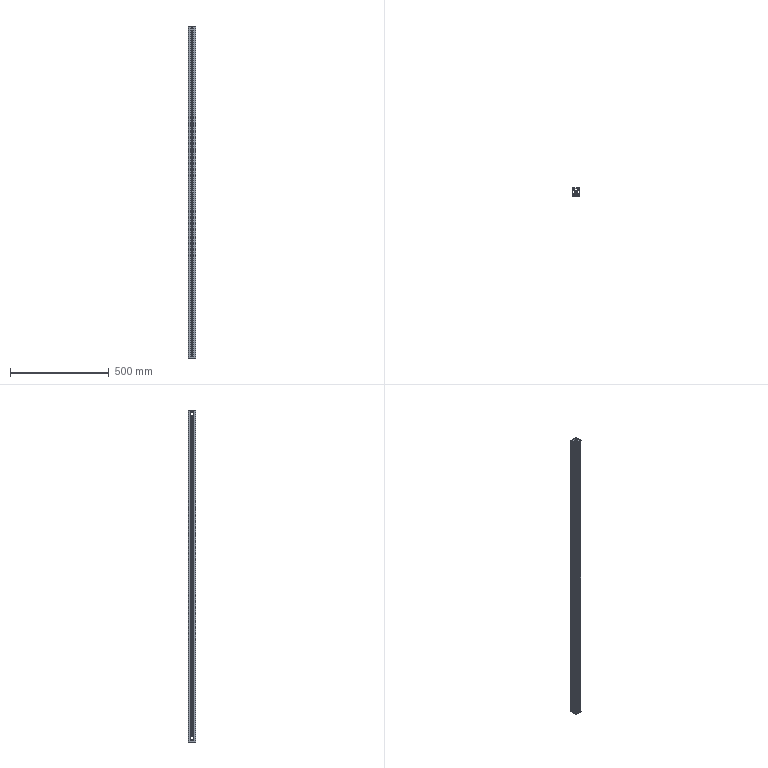Part | SolidWorks | features BaseBody 1, HoleWzd 1, MoveFace 1 | 1 solid | 242 faces | box 40 x 40 x 1682 mm | volume 987483 mm3 | plane 187 | cylinder 55 | commonest cylinder face diameters 6.8 x15 2 x14 19 x12 1 x6 5 x4 9 x4